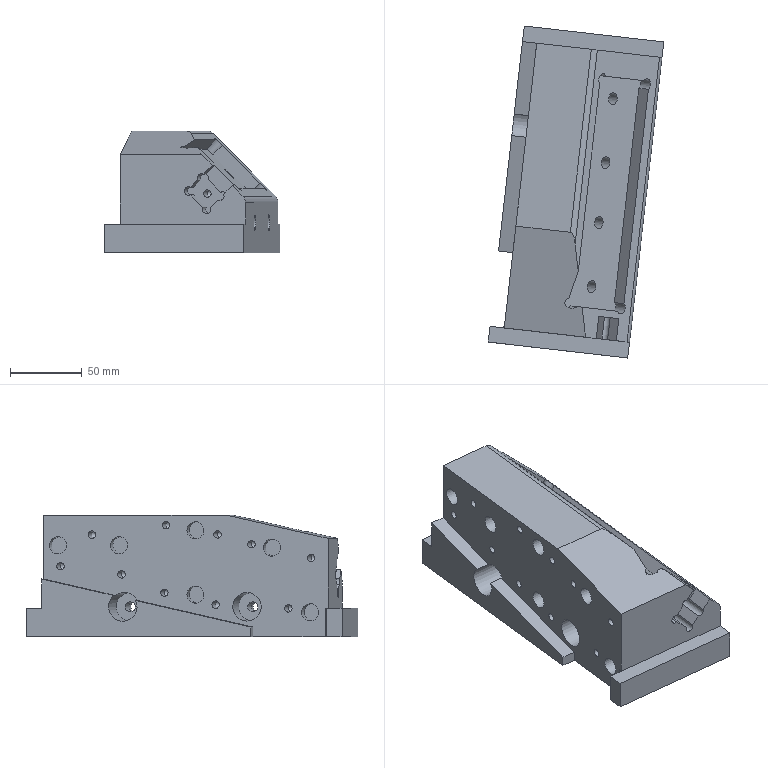Part | NX | features XQ 2 | 1 solid | 94 faces | box 122.501 x 231.667 x 85 mm | volume 1183621 mm3 | plane 41 | cylinder 38 | cone 15 | commonest cylinder face diameters 5.2 x11 12 x8 6 x4 8 x4 8.5 x4 7 x2